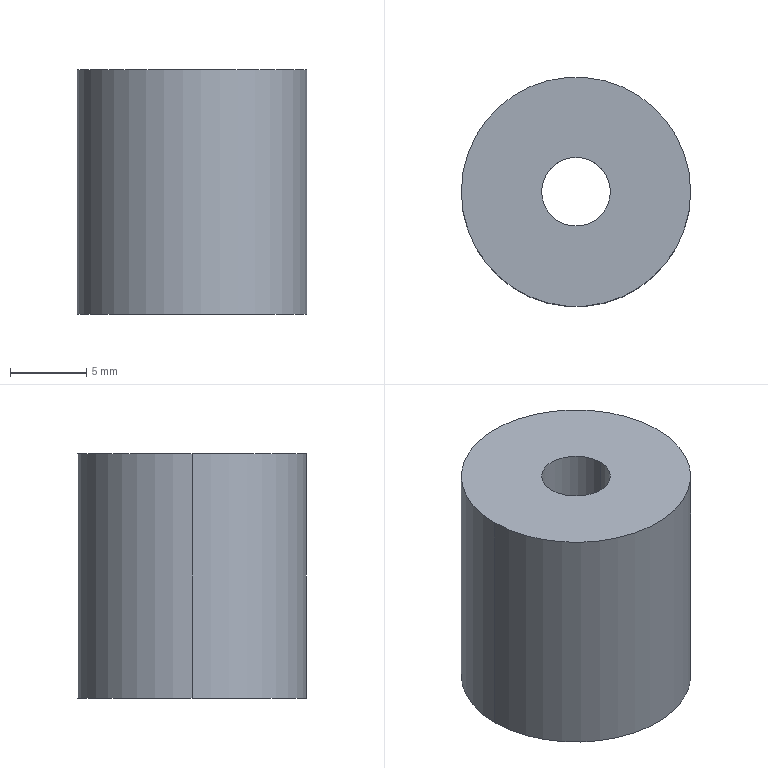Part | SolidWorks | features Chamfer 1, Extrusion 1, HoleWzd 1 | 1 solid | 11 faces | box 15 x 15 x 16 mm | volume 1985 mm3 | cylinder 6 | plane 3 | cone 2 | commonest cylinder face diameters 4.5 x2 9 x2 15 x2
STEP:
#1=CARTESIAN_POINT('',(4.5,0.,1.));
#2=VERTEX_POINT('',#1);
#3=CARTESIAN_POINT('',(-4.5,0.,1.));
#4=VERTEX_POINT('',#3);
#5=CARTESIAN_POINT('',(0.,0.,1.));
#6=DIRECTION('',(0.,0.,-1.));
#7=DIRECTION('',(1.,0.,0.));
#8=AXIS2_PLACEMENT_3D('',#5,#6,#7);
#9=CIRCLE('',#8,4.5);
#10=EDGE_CURVE('',#2,#4,#9,.T.);
#11=ORIENTED_EDGE('',*,*,#10,.F.);
#12=CARTESIAN_POINT('',(5.5,0.,0.));
#13=VERTEX_POINT('',#12);
#14=CARTESIAN_POINT('',(4.5,0.,1.));
#15=DIRECTION('',(0.7071,0.,-0.7071));
#16=VECTOR('',#15,1000.);
#17=LINE('',#14,#16);
#18=EDGE_CURVE('',#2,#13,#17,.T.);
#19=ORIENTED_EDGE('',*,*,#18,.T.);
#20=CARTESIAN_POINT('',(-5.5,0.,0.));
#21=VERTEX_POINT('',#20);
#22=CARTESIAN_POINT('',(0.,0.,0.));
#23=DIRECTION('',(0.,0.,1.));
#24=DIRECTION('',(1.,0.,0.));
#25=AXIS2_PLACEMENT_3D('',#22,#23,#24);
#26=CIRCLE('',#25,5.5);
#27=EDGE_CURVE('',#21,#13,#26,.T.);
#28=ORIENTED_EDGE('',*,*,#27,.F.);
#29=CARTESIAN_POINT('',(-4.5,0.,1.));
#30=DIRECTION('',(-0.7071,0.,-0.7071));
#31=VECTOR('',#30,1000.);
#32=LINE('',#29,#31);
#33=EDGE_CURVE('',#4,#21,#32,.T.);
#34=ORIENTED_EDGE('',*,*,#33,.F.);
#35=EDGE_LOOP('',(#11,#19,#28,#34));
#36=FACE_OUTER_BOUND('',#35,.T.);
#37=CARTESIAN_POINT('',(0.,0.,1.));
#38=DIRECTION('',(0.,0.,-1.));
#39=DIRECTION('',(-1.,0.,0.));
#40=AXIS2_PLACEMENT_3D('',#37,#38,#39);
#41=CONICAL_SURFACE('',#40,4.5,0.7854);
#42=ADVANCED_FACE('',(#36),#41,.F.);
#43=CARTESIAN_POINT('',(4.5,0.,12.));
#44=VERTEX_POINT('',#43);
#45=CARTESIAN_POINT('',(-4.5,0.,12.));
#46=VERTEX_POINT('',#45);
#47=CARTESIAN_POINT('',(0.,0.,12.));
#48=DIRECTION('',(0.,0.,-1.));
#49=DIRECTION('',(-1.,0.,0.));
#50=AXIS2_PLACEMENT_3D('',#47,#48,#49);
#51=CIRCLE('',#50,4.5);
#52=EDGE_CURVE('',#44,#46,#51,.T.);
#53=ORIENTED_EDGE('',*,*,#52,.F.);
#54=CARTESIAN_POINT('',(4.5,0.,0.));
#55=DIRECTION('',(0.,0.,-1.));
#56=VECTOR('',#55,1000.);
#57=LINE('',#54,#56);
#58=EDGE_CURVE('',#44,#2,#57,.T.);
#59=ORIENTED_EDGE('',*,*,#58,.T.);
#60=ORIENTED_EDGE('',*,*,#10,.T.);
#61=CARTESIAN_POINT('',(-4.5,0.,0.));
#62=DIRECTION('',(0.,0.,-1.));
#63=VECTOR('',#62,1000.);
#64=LINE('',#61,#63);
#65=EDGE_CURVE('',#46,#4,#64,.T.);
#66=ORIENTED_EDGE('',*,*,#65,.F.);
#67=EDGE_LOOP('',(#53,#59,#60,#66));
#68=FACE_OUTER_BOUND('',#67,.T.);
#69=CARTESIAN_POINT('',(0.,0.,0.));
#70=DIRECTION('',(0.,0.,-1.));
#71=DIRECTION('',(-1.,0.,0.));
#72=AXIS2_PLACEMENT_3D('',#69,#70,#71);
#73=CYLINDRICAL_SURFACE('',#72,4.5);
#74=ADVANCED_FACE('',(#68),#73,.F.);
#75=CARTESIAN_POINT('',(2.25,0.,16.));
#76=VERTEX_POINT('',#75);
#77=CARTESIAN_POINT('',(-2.25,0.,16.));
#78=VERTEX_POINT('',#77);
#79=CARTESIAN_POINT('',(0.,0.,16.));
#80=DIRECTION('',(0.,0.,-1.));
#81=DIRECTION('',(-1.,0.,0.));
#82=AXIS2_PLACEMENT_3D('',#79,#80,#81);
#83=CIRCLE('',#82,2.25);
#84=EDGE_CURVE('',#76,#78,#83,.T.);
#85=ORIENTED_EDGE('',*,*,#84,.F.);
#86=CARTESIAN_POINT('',(2.25,0.,12.));
#87=VERTEX_POINT('',#86);
#88=CARTESIAN_POINT('',(2.25,0.,0.));
#89=DIRECTION('',(0.,0.,-1.));
#90=VECTOR('',#89,1000.);
#91=LINE('',#88,#90);
#92=EDGE_CURVE('',#76,#87,#91,.T.);
#93=ORIENTED_EDGE('',*,*,#92,.T.);
#94=CARTESIAN_POINT('',(-2.25,0.,12.));
#95=VERTEX_POINT('',#94);
#96=CARTESIAN_POINT('',(0.,0.,12.));
#97=DIRECTION('',(0.,0.,-1.));
#98=DIRECTION('',(-1.,0.,0.));
#99=AXIS2_PLACEMENT_3D('',#96,#97,#98);
#100=CIRCLE('',#99,2.25);
#101=EDGE_CURVE('',#87,#95,#100,.T.);
#102=ORIENTED_EDGE('',*,*,#101,.T.);
#103=CARTESIAN_POINT('',(-2.25,0.,0.));
#104=DIRECTION('',(0.,0.,-1.));
#105=VECTOR('',#104,1000.);
#106=LINE('',#103,#105);
#107=EDGE_CURVE('',#78,#95,#106,.T.);
#108=ORIENTED_EDGE('',*,*,#107,.F.);
#109=EDGE_LOOP('',(#85,#93,#102,#108));
#110=FACE_OUTER_BOUND('',#109,.T.);
#111=CARTESIAN_POINT('',(0.,0.,0.));
#112=DIRECTION('',(0.,0.,-1.));
#113=DIRECTION('',(-1.,0.,0.));
#114=AXIS2_PLACEMENT_3D('',#111,#112,#113);
#115=CYLINDRICAL_SURFACE('',#114,2.25);
#116=ADVANCED_FACE('',(#110),#115,.F.);
#117=CARTESIAN_POINT('',(7.5,0.,16.));
#118=VERTEX_POINT('',#117);
#119=CARTESIAN_POINT('',(-7.5,0.,16.));
#120=VERTEX_POINT('',#119);
#121=CARTESIAN_POINT('',(0.,0.,16.));
#122=DIRECTION('',(0.,0.,1.));
#123=DIRECTION('',(1.,0.,0.));
#124=AXIS2_PLACEMENT_3D('',#121,#122,#123);
#125=CIRCLE('',#124,7.5);
#126=EDGE_CURVE('',#118,#120,#125,.T.);
#127=ORIENTED_EDGE('',*,*,#126,.F.);
#128=CARTESIAN_POINT('',(7.5,0.,0.));
#129=VERTEX_POINT('',#128);
#130=CARTESIAN_POINT('',(7.5,0.,16.));
#131=DIRECTION('',(0.,0.,-1.));
#132=VECTOR('',#131,1000.);
#133=LINE('',#130,#132);
#134=EDGE_CURVE('',#118,#129,#133,.T.);
#135=ORIENTED_EDGE('',*,*,#134,.T.);
#136=CARTESIAN_POINT('',(-7.5,0.,0.));
#137=VERTEX_POINT('',#136);
#138=CARTESIAN_POINT('',(0.,0.,0.));
#139=DIRECTION('',(0.,0.,1.));
#140=DIRECTION('',(1.,0.,0.));
#141=AXIS2_PLACEMENT_3D('',#138,#139,#140);
#142=CIRCLE('',#141,7.5);
#143=EDGE_CURVE('',#129,#137,#142,.T.);
#144=ORIENTED_EDGE('',*,*,#143,.T.);
#145=CARTESIAN_POINT('',(-7.5,0.,16.));
#146=DIRECTION('',(0.,0.,-1.));
#147=VECTOR('',#146,1000.);
#148=LINE('',#145,#147);
#149=EDGE_CURVE('',#120,#137,#148,.T.);
#150=ORIENTED_EDGE('',*,*,#149,.F.);
#151=EDGE_LOOP('',(#127,#135,#144,#150));
#152=FACE_OUTER_BOUND('',#151,.T.);
#153=CARTESIAN_POINT('',(0.,0.,16.));
#154=DIRECTION('',(0.,0.,-1.));
#155=DIRECTION('',(-1.,0.,0.));
#156=AXIS2_PLACEMENT_3D('',#153,#154,#155);
#157=CYLINDRICAL_SURFACE('',#156,7.5);
#158=ADVANCED_FACE('',(#152),#157,.T.);
#159=ORIENTED_EDGE('',*,*,#134,.F.);
#160=CARTESIAN_POINT('',(0.,0.,16.));
#161=DIRECTION('',(0.,0.,1.));
#162=DIRECTION('',(1.,0.,0.));
#163=AXIS2_PLACEMENT_3D('',#160,#161,#162);
#164=CIRCLE('',#163,7.5);
#165=EDGE_CURVE('',#120,#118,#164,.T.);
#166=ORIENTED_EDGE('',*,*,#165,.F.);
#167=ORIENTED_EDGE('',*,*,#149,.T.);
#168=CARTESIAN_POINT('',(0.,0.,0.));
#169=DIRECTION('',(0.,0.,1.));
#170=DIRECTION('',(1.,0.,0.));
#171=AXIS2_PLACEMENT_3D('',#168,#169,#170);
#172=CIRCLE('',#171,7.5);
#173=EDGE_CURVE('',#137,#129,#172,.T.);
#174=ORIENTED_EDGE('',*,*,#173,.T.);
#175=EDGE_LOOP('',(#159,#166,#167,#174));
#176=FACE_OUTER_BOUND('',#175,.T.);
#177=CARTESIAN_POINT('',(0.,0.,16.));
#178=DIRECTION('',(0.,0.,-1.));
#179=DIRECTION('',(-1.,0.,0.));
#180=AXIS2_PLACEMENT_3D('',#177,#178,#179);
#181=CYLINDRICAL_SURFACE('',#180,7.5);
#182=ADVANCED_FACE('',(#176),#181,.T.);
#183=CARTESIAN_POINT('',(0.,0.,16.));
#184=DIRECTION('',(0.,0.,-1.));
#185=DIRECTION('',(-1.,0.,0.));
#186=AXIS2_PLACEMENT_3D('',#183,#184,#185);
#187=CIRCLE('',#186,2.25);
#188=EDGE_CURVE('',#78,#76,#187,.T.);
#189=ORIENTED_EDGE('',*,*,#188,.T.);
#190=ORIENTED_EDGE('',*,*,#84,.T.);
#191=EDGE_LOOP('',(#189,#190));
#192=FACE_BOUND('',#191,.T.);
#193=ORIENTED_EDGE('',*,*,#165,.T.);
#194=ORIENTED_EDGE('',*,*,#126,.T.);
#195=EDGE_LOOP('',(#193,#194));
#196=FACE_OUTER_BOUND('',#195,.T.);
#197=CARTESIAN_POINT('',(0.,0.,16.));
#198=DIRECTION('',(0.,0.,1.));
#199=DIRECTION('',(1.,0.,0.));
#200=AXIS2_PLACEMENT_3D('',#197,#198,#199);
#201=PLANE('',#200);
#202=ADVANCED_FACE('',(#192,#196),#201,.T.);
#203=ORIENTED_EDGE('',*,*,#27,.T.);
#204=CARTESIAN_POINT('',(0.,0.,0.));
#205=DIRECTION('',(0.,0.,1.));
#206=DIRECTION('',(1.,0.,0.));
#207=AXIS2_PLACEMENT_3D('',#204,#205,#206);
#208=CIRCLE('',#207,5.5);
#209=EDGE_CURVE('',#13,#21,#208,.T.);
#210=ORIENTED_EDGE('',*,*,#209,.T.);
#211=EDGE_LOOP('',(#203,#210));
#212=FACE_BOUND('',#211,.T.);
#213=ORIENTED_EDGE('',*,*,#173,.F.);
#214=ORIENTED_EDGE('',*,*,#143,.F.);
#215=EDGE_LOOP('',(#213,#214));
#216=FACE_OUTER_BOUND('',#215,.T.);
#217=CARTESIAN_POINT('',(0.,0.,0.));
#218=DIRECTION('',(0.,0.,1.));
#219=DIRECTION('',(1.,0.,0.));
#220=AXIS2_PLACEMENT_3D('',#217,#218,#219);
#221=PLANE('',#220);
#222=ADVANCED_FACE('',(#212,#216),#221,.F.);
#223=ORIENTED_EDGE('',*,*,#92,.F.);
#224=ORIENTED_EDGE('',*,*,#188,.F.);
#225=ORIENTED_EDGE('',*,*,#107,.T.);
#226=CARTESIAN_POINT('',(0.,0.,12.));
#227=DIRECTION('',(0.,0.,-1.));
#228=DIRECTION('',(-1.,0.,0.));
#229=AXIS2_PLACEMENT_3D('',#226,#227,#228);
#230=CIRCLE('',#229,2.25);
#231=EDGE_CURVE('',#95,#87,#230,.T.);
#232=ORIENTED_EDGE('',*,*,#231,.T.);
#233=EDGE_LOOP('',(#223,#224,#225,#232));
#234=FACE_OUTER_BOUND('',#233,.T.);
#235=CARTESIAN_POINT('',(0.,0.,0.));
#236=DIRECTION('',(0.,0.,-1.));
#237=DIRECTION('',(-1.,0.,0.));
#238=AXIS2_PLACEMENT_3D('',#235,#236,#237);
#239=CYLINDRICAL_SURFACE('',#238,2.25);
#240=ADVANCED_FACE('',(#234),#239,.F.);
#241=ORIENTED_EDGE('',*,*,#231,.F.);
#242=ORIENTED_EDGE('',*,*,#101,.F.);
#243=EDGE_LOOP('',(#241,#242));
#244=FACE_BOUND('',#243,.T.);
#245=CARTESIAN_POINT('',(0.,0.,12.));
#246=DIRECTION('',(0.,0.,-1.));
#247=DIRECTION('',(-1.,0.,0.));
#248=AXIS2_PLACEMENT_3D('',#245,#246,#247);
#249=CIRCLE('',#248,4.5);
#250=EDGE_CURVE('',#46,#44,#249,.T.);
#251=ORIENTED_EDGE('',*,*,#250,.T.);
#252=ORIENTED_EDGE('',*,*,#52,.T.);
#253=EDGE_LOOP('',(#251,#252));
#254=FACE_OUTER_BOUND('',#253,.T.);
#255=CARTESIAN_POINT('',(2.25,0.,12.));
#256=DIRECTION('',(0.,0.,1.));
#257=DIRECTION('',(1.,0.,0.));
#258=AXIS2_PLACEMENT_3D('',#255,#256,#257);
#259=PLANE('',#258);
#260=ADVANCED_FACE('',(#244,#254),#259,.F.);
#261=ORIENTED_EDGE('',*,*,#58,.F.);
#262=ORIENTED_EDGE('',*,*,#250,.F.);
#263=ORIENTED_EDGE('',*,*,#65,.T.);
#264=CARTESIAN_POINT('',(0.,0.,1.));
#265=DIRECTION('',(0.,0.,-1.));
#266=DIRECTION('',(1.,0.,0.));
#267=AXIS2_PLACEMENT_3D('',#264,#265,#266);
#268=CIRCLE('',#267,4.5);
#269=EDGE_CURVE('',#4,#2,#268,.T.);
#270=ORIENTED_EDGE('',*,*,#269,.T.);
#271=EDGE_LOOP('',(#261,#262,#263,#270));
#272=FACE_OUTER_BOUND('',#271,.T.);
#273=CARTESIAN_POINT('',(0.,0.,0.));
#274=DIRECTION('',(0.,0.,-1.));
#275=DIRECTION('',(-1.,0.,0.));
#276=AXIS2_PLACEMENT_3D('',#273,#274,#275);
#277=CYLINDRICAL_SURFACE('',#276,4.5);
#278=ADVANCED_FACE('',(#272),#277,.F.);
#279=ORIENTED_EDGE('',*,*,#18,.F.);
#280=ORIENTED_EDGE('',*,*,#269,.F.);
#281=ORIENTED_EDGE('',*,*,#33,.T.);
#282=ORIENTED_EDGE('',*,*,#209,.F.);
#283=EDGE_LOOP('',(#279,#280,#281,#282));
#284=FACE_OUTER_BOUND('',#283,.T.);
#285=CARTESIAN_POINT('',(0.,0.,1.));
#286=DIRECTION('',(0.,0.,-1.));
#287=DIRECTION('',(-1.,0.,0.));
#288=AXIS2_PLACEMENT_3D('',#285,#286,#287);
#289=CONICAL_SURFACE('',#288,4.5,0.7854);
#290=ADVANCED_FACE('',(#284),#289,.F.);
#291=CLOSED_SHELL('',(#42,#74,#116,#158,#182,#202,#222,#240,#260,#278,#290));
#292=MANIFOLD_SOLID_BREP('',#291);
#293=CARTESIAN_POINT('',(0.,0.,0.));
#294=DIRECTION('',(0.,0.,1.));
#295=DIRECTION('',(1.,0.,0.));
#296=AXIS2_PLACEMENT_3D('',#293,#294,#295);
#297=(LENGTH_UNIT()NAMED_UNIT(*)SI_UNIT(.MILLI.,.METRE.));
#298=UNCERTAINTY_MEASURE_WITH_UNIT(LENGTH_MEASURE(0.00001),#297,'','');
#299=(NAMED_UNIT(*)PLANE_ANGLE_UNIT()SI_UNIT($,.RADIAN.));
#300=(NAMED_UNIT(*)SI_UNIT($,.STERADIAN.)SOLID_ANGLE_UNIT());
#301=(GEOMETRIC_REPRESENTATION_CONTEXT(3)GLOBAL_UNCERTAINTY_ASSIGNED_CONTEXT((#298))GLOBAL_UNIT_ASSIGNED_CONTEXT((#297,#299,#300))REPRESENTATION_CONTEXT('',''));
#302=ADVANCED_BREP_SHAPE_REPRESENTATION('',(#292,#296),#301);